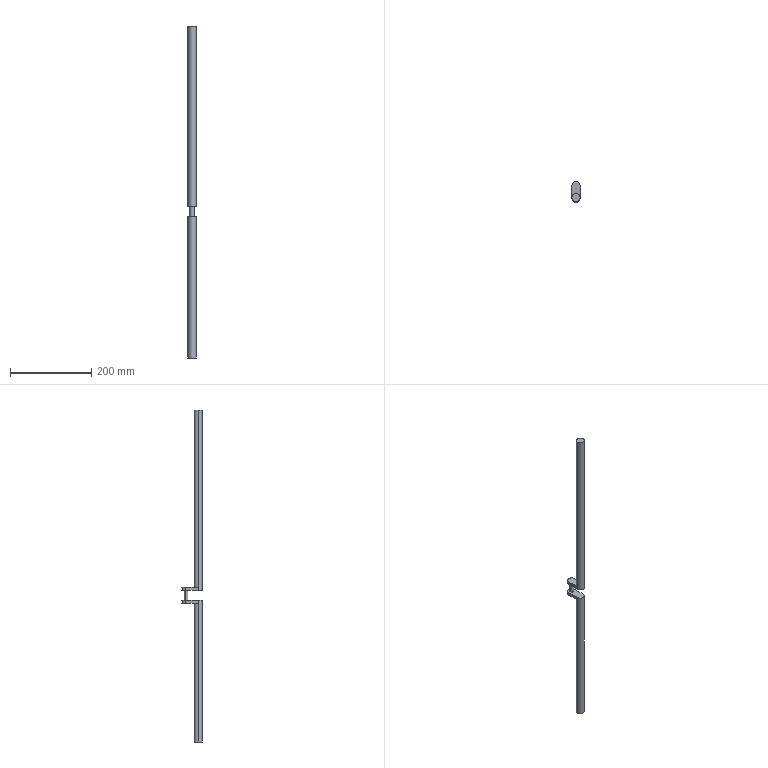Part | SolidWorks | features ICE 5, Extrusion 1 | 1 solid | 18 faces | box 20 x 50 x 819.2 mm | volume 260469 mm3 | plane 10 | cylinder 8 | commonest cylinder face diameters 20 x6 10 x2
STEP:
#1=CARTESIAN_POINT('',(10.,0.,457.2));
#2=VERTEX_POINT('',#1);
#3=CARTESIAN_POINT('',(-10.,0.,457.2));
#4=VERTEX_POINT('',#3);
#5=CARTESIAN_POINT('',(0.,0.,457.2));
#6=DIRECTION('',(0.,0.,1.));
#7=DIRECTION('',(1.,0.,0.));
#8=AXIS2_PLACEMENT_3D('',#5,#6,#7);
#9=CIRCLE('',#8,10.);
#10=EDGE_CURVE('',#2,#4,#9,.T.);
#11=ORIENTED_EDGE('',*,*,#10,.F.);
#12=CARTESIAN_POINT('',(10.,0.,20.));
#13=VERTEX_POINT('',#12);
#14=CARTESIAN_POINT('',(10.,0.,362.));
#15=DIRECTION('',(0.,0.,-1.));
#16=VECTOR('',#15,1000.);
#17=LINE('',#14,#16);
#18=EDGE_CURVE('',#2,#13,#17,.T.);
#19=ORIENTED_EDGE('',*,*,#18,.T.);
#20=CARTESIAN_POINT('',(-10.,0.,20.));
#21=VERTEX_POINT('',#20);
#22=CARTESIAN_POINT('',(0.,0.,20.));
#23=DIRECTION('',(0.,0.,1.));
#24=DIRECTION('',(1.,0.,0.));
#25=AXIS2_PLACEMENT_3D('',#22,#23,#24);
#26=CIRCLE('',#25,10.);
#27=EDGE_CURVE('',#13,#21,#26,.T.);
#28=ORIENTED_EDGE('',*,*,#27,.T.);
#29=CARTESIAN_POINT('',(-10.,0.,362.));
#30=DIRECTION('',(0.,0.,-1.));
#31=VECTOR('',#30,1000.);
#32=LINE('',#29,#31);
#33=EDGE_CURVE('',#4,#21,#32,.T.);
#34=ORIENTED_EDGE('',*,*,#33,.F.);
#35=EDGE_LOOP('',(#11,#19,#28,#34));
#36=FACE_OUTER_BOUND('',#35,.T.);
#37=CARTESIAN_POINT('',(0.,0.,362.));
#38=DIRECTION('',(0.,0.,-1.));
#39=DIRECTION('',(-1.,0.,0.));
#40=AXIS2_PLACEMENT_3D('',#37,#38,#39);
#41=CYLINDRICAL_SURFACE('',#40,10.);
#42=ADVANCED_FACE('',(#36),#41,.T.);
#43=CARTESIAN_POINT('',(5.,30.,12.5));
#44=VERTEX_POINT('',#43);
#45=CARTESIAN_POINT('',(-5.,30.,12.5));
#46=VERTEX_POINT('',#45);
#47=CARTESIAN_POINT('',(0.,30.,12.5));
#48=DIRECTION('',(0.,0.,1.));
#49=DIRECTION('',(1.,0.,0.));
#50=AXIS2_PLACEMENT_3D('',#47,#48,#49);
#51=CIRCLE('',#50,5.);
#52=EDGE_CURVE('',#44,#46,#51,.T.);
#53=ORIENTED_EDGE('',*,*,#52,.F.);
#54=CARTESIAN_POINT('',(5.,30.,-12.5));
#55=VERTEX_POINT('',#54);
#56=CARTESIAN_POINT('',(5.,30.,12.5));
#57=DIRECTION('',(0.,0.,-1.));
#58=VECTOR('',#57,1000.);
#59=LINE('',#56,#58);
#60=EDGE_CURVE('',#44,#55,#59,.T.);
#61=ORIENTED_EDGE('',*,*,#60,.T.);
#62=CARTESIAN_POINT('',(-5.,30.,-12.5));
#63=VERTEX_POINT('',#62);
#64=CARTESIAN_POINT('',(0.,30.,-12.5));
#65=DIRECTION('',(0.,0.,1.));
#66=DIRECTION('',(-1.,0.,0.));
#67=AXIS2_PLACEMENT_3D('',#64,#65,#66);
#68=CIRCLE('',#67,5.);
#69=EDGE_CURVE('',#55,#63,#68,.T.);
#70=ORIENTED_EDGE('',*,*,#69,.T.);
#71=CARTESIAN_POINT('',(-5.,30.,12.5));
#72=DIRECTION('',(0.,0.,-1.));
#73=VECTOR('',#72,1000.);
#74=LINE('',#71,#73);
#75=EDGE_CURVE('',#46,#63,#74,.T.);
#76=ORIENTED_EDGE('',*,*,#75,.F.);
#77=EDGE_LOOP('',(#53,#61,#70,#76));
#78=FACE_OUTER_BOUND('',#77,.T.);
#79=CARTESIAN_POINT('',(0.,30.,12.5));
#80=DIRECTION('',(0.,0.,-1.));
#81=DIRECTION('',(-1.,0.,0.));
#82=AXIS2_PLACEMENT_3D('',#79,#80,#81);
#83=CYLINDRICAL_SURFACE('',#82,5.);
#84=ADVANCED_FACE('',(#78),#83,.T.);
#85=CARTESIAN_POINT('',(-10.,0.,-20.));
#86=VERTEX_POINT('',#85);
#87=CARTESIAN_POINT('',(10.,0.,-20.));
#88=VERTEX_POINT('',#87);
#89=CARTESIAN_POINT('',(0.,0.,-20.));
#90=DIRECTION('',(0.,0.,-1.));
#91=DIRECTION('',(-1.,0.,0.));
#92=AXIS2_PLACEMENT_3D('',#89,#90,#91);
#93=CIRCLE('',#92,10.);
#94=EDGE_CURVE('',#86,#88,#93,.T.);
#95=ORIENTED_EDGE('',*,*,#94,.T.);
#96=CARTESIAN_POINT('',(10.,0.,-362.));
#97=VERTEX_POINT('',#96);
#98=CARTESIAN_POINT('',(10.,0.,362.));
#99=DIRECTION('',(0.,0.,-1.));
#100=VECTOR('',#99,1000.);
#101=LINE('',#98,#100);
#102=EDGE_CURVE('',#88,#97,#101,.T.);
#103=ORIENTED_EDGE('',*,*,#102,.T.);
#104=CARTESIAN_POINT('',(-10.,0.,-362.));
#105=VERTEX_POINT('',#104);
#106=CARTESIAN_POINT('',(0.,0.,-362.));
#107=DIRECTION('',(0.,0.,1.));
#108=DIRECTION('',(1.,0.,0.));
#109=AXIS2_PLACEMENT_3D('',#106,#107,#108);
#110=CIRCLE('',#109,10.);
#111=EDGE_CURVE('',#97,#105,#110,.T.);
#112=ORIENTED_EDGE('',*,*,#111,.T.);
#113=CARTESIAN_POINT('',(-10.,0.,362.));
#114=DIRECTION('',(0.,0.,-1.));
#115=VECTOR('',#114,1000.);
#116=LINE('',#113,#115);
#117=EDGE_CURVE('',#86,#105,#116,.T.);
#118=ORIENTED_EDGE('',*,*,#117,.F.);
#119=EDGE_LOOP('',(#95,#103,#112,#118));
#120=FACE_OUTER_BOUND('',#119,.T.);
#121=CARTESIAN_POINT('',(0.,0.,362.));
#122=DIRECTION('',(0.,0.,-1.));
#123=DIRECTION('',(-1.,0.,0.));
#124=AXIS2_PLACEMENT_3D('',#121,#122,#123);
#125=CYLINDRICAL_SURFACE('',#124,10.);
#126=ADVANCED_FACE('',(#120),#125,.T.);
#127=ORIENTED_EDGE('',*,*,#102,.F.);
#128=CARTESIAN_POINT('',(10.,0.,-12.5));
#129=VERTEX_POINT('',#128);
#130=CARTESIAN_POINT('',(10.,0.,20.));
#131=DIRECTION('',(0.,0.,-1.));
#132=VECTOR('',#131,1000.);
#133=LINE('',#130,#132);
#134=EDGE_CURVE('',#129,#88,#133,.T.);
#135=ORIENTED_EDGE('',*,*,#134,.F.);
#136=CARTESIAN_POINT('',(-10.,0.,-12.5));
#137=VERTEX_POINT('',#136);
#138=CARTESIAN_POINT('',(0.,0.,-12.5));
#139=DIRECTION('',(0.,0.,-1.));
#140=DIRECTION('',(-1.,0.,0.));
#141=AXIS2_PLACEMENT_3D('',#138,#139,#140);
#142=CIRCLE('',#141,10.);
#143=EDGE_CURVE('',#129,#137,#142,.T.);
#144=ORIENTED_EDGE('',*,*,#143,.T.);
#145=CARTESIAN_POINT('',(-10.,0.,20.));
#146=DIRECTION('',(0.,0.,-1.));
#147=VECTOR('',#146,1000.);
#148=LINE('',#145,#147);
#149=EDGE_CURVE('',#137,#86,#148,.T.);
#150=ORIENTED_EDGE('',*,*,#149,.T.);
#151=ORIENTED_EDGE('',*,*,#117,.T.);
#152=CARTESIAN_POINT('',(0.,0.,-362.));
#153=DIRECTION('',(0.,0.,1.));
#154=DIRECTION('',(1.,0.,0.));
#155=AXIS2_PLACEMENT_3D('',#152,#153,#154);
#156=CIRCLE('',#155,10.);
#157=EDGE_CURVE('',#105,#97,#156,.T.);
#158=ORIENTED_EDGE('',*,*,#157,.T.);
#159=EDGE_LOOP('',(#127,#135,#144,#150,#151,#158));
#160=FACE_OUTER_BOUND('',#159,.T.);
#161=CARTESIAN_POINT('',(0.,0.,362.));
#162=DIRECTION('',(0.,0.,-1.));
#163=DIRECTION('',(-1.,0.,0.));
#164=AXIS2_PLACEMENT_3D('',#161,#162,#163);
#165=CYLINDRICAL_SURFACE('',#164,10.);
#166=ADVANCED_FACE('',(#160),#165,.T.);
#167=CARTESIAN_POINT('',(10.,30.,-12.5));
#168=VERTEX_POINT('',#167);
#169=CARTESIAN_POINT('',(10.,30.,-20.));
#170=VERTEX_POINT('',#169);
#171=CARTESIAN_POINT('',(10.,30.,20.));
#172=DIRECTION('',(0.,0.,-1.));
#173=VECTOR('',#172,1000.);
#174=LINE('',#171,#173);
#175=EDGE_CURVE('',#168,#170,#174,.T.);
#176=ORIENTED_EDGE('',*,*,#175,.F.);
#177=CARTESIAN_POINT('',(10.,0.,-12.5));
#178=DIRECTION('',(0.,-1.,0.));
#179=VECTOR('',#178,1000.);
#180=LINE('',#177,#179);
#181=EDGE_CURVE('',#168,#129,#180,.T.);
#182=ORIENTED_EDGE('',*,*,#181,.T.);
#183=ORIENTED_EDGE('',*,*,#134,.T.);
#184=CARTESIAN_POINT('',(10.,0.,-20.));
#185=DIRECTION('',(0.,1.,0.));
#186=VECTOR('',#185,1000.);
#187=LINE('',#184,#186);
#188=EDGE_CURVE('',#88,#170,#187,.T.);
#189=ORIENTED_EDGE('',*,*,#188,.T.);
#190=EDGE_LOOP('',(#176,#182,#183,#189));
#191=FACE_OUTER_BOUND('',#190,.T.);
#192=CARTESIAN_POINT('',(10.,0.,20.));
#193=DIRECTION('',(-1.,0.,0.));
#194=DIRECTION('',(0.,0.,1.));
#195=AXIS2_PLACEMENT_3D('',#192,#193,#194);
#196=PLANE('',#195);
#197=ADVANCED_FACE('',(#191),#196,.F.);
#198=CARTESIAN_POINT('',(-10.,30.,-12.5));
#199=VERTEX_POINT('',#198);
#200=CARTESIAN_POINT('',(-10.,30.,-20.));
#201=VERTEX_POINT('',#200);
#202=CARTESIAN_POINT('',(-10.,30.,20.));
#203=DIRECTION('',(0.,0.,-1.));
#204=VECTOR('',#203,1000.);
#205=LINE('',#202,#204);
#206=EDGE_CURVE('',#199,#201,#205,.T.);
#207=ORIENTED_EDGE('',*,*,#206,.F.);
#208=CARTESIAN_POINT('',(0.,30.,-12.5));
#209=DIRECTION('',(0.,0.,-1.));
#210=DIRECTION('',(-1.,0.,0.));
#211=AXIS2_PLACEMENT_3D('',#208,#209,#210);
#212=CIRCLE('',#211,10.);
#213=EDGE_CURVE('',#199,#168,#212,.T.);
#214=ORIENTED_EDGE('',*,*,#213,.T.);
#215=ORIENTED_EDGE('',*,*,#175,.T.);
#216=CARTESIAN_POINT('',(0.,30.,-20.));
#217=DIRECTION('',(0.,0.,1.));
#218=DIRECTION('',(1.,0.,0.));
#219=AXIS2_PLACEMENT_3D('',#216,#217,#218);
#220=CIRCLE('',#219,10.);
#221=EDGE_CURVE('',#170,#201,#220,.T.);
#222=ORIENTED_EDGE('',*,*,#221,.T.);
#223=EDGE_LOOP('',(#207,#214,#215,#222));
#224=FACE_OUTER_BOUND('',#223,.T.);
#225=CARTESIAN_POINT('',(0.,30.,20.));
#226=DIRECTION('',(0.,0.,-1.));
#227=DIRECTION('',(-1.,0.,0.));
#228=AXIS2_PLACEMENT_3D('',#225,#226,#227);
#229=CYLINDRICAL_SURFACE('',#228,10.);
#230=ADVANCED_FACE('',(#224),#229,.T.);
#231=ORIENTED_EDGE('',*,*,#149,.F.);
#232=CARTESIAN_POINT('',(-10.,0.,-12.5));
#233=DIRECTION('',(0.,1.,0.));
#234=VECTOR('',#233,1000.);
#235=LINE('',#232,#234);
#236=EDGE_CURVE('',#137,#199,#235,.T.);
#237=ORIENTED_EDGE('',*,*,#236,.T.);
#238=ORIENTED_EDGE('',*,*,#206,.T.);
#239=CARTESIAN_POINT('',(-10.,0.,-20.));
#240=DIRECTION('',(0.,-1.,0.));
#241=VECTOR('',#240,1000.);
#242=LINE('',#239,#241);
#243=EDGE_CURVE('',#201,#86,#242,.T.);
#244=ORIENTED_EDGE('',*,*,#243,.T.);
#245=EDGE_LOOP('',(#231,#237,#238,#244));
#246=FACE_OUTER_BOUND('',#245,.T.);
#247=CARTESIAN_POINT('',(-10.,0.,20.));
#248=DIRECTION('',(1.,0.,0.));
#249=DIRECTION('',(0.,0.,-1.));
#250=AXIS2_PLACEMENT_3D('',#247,#248,#249);
#251=PLANE('',#250);
#252=ADVANCED_FACE('',(#246),#251,.F.);
#253=ORIENTED_EDGE('',*,*,#94,.F.);
#254=ORIENTED_EDGE('',*,*,#243,.F.);
#255=ORIENTED_EDGE('',*,*,#221,.F.);
#256=ORIENTED_EDGE('',*,*,#188,.F.);
#257=EDGE_LOOP('',(#253,#254,#255,#256));
#258=FACE_OUTER_BOUND('',#257,.T.);
#259=CARTESIAN_POINT('',(0.,0.,-20.));
#260=DIRECTION('',(0.,0.,1.));
#261=DIRECTION('',(1.,0.,0.));
#262=AXIS2_PLACEMENT_3D('',#259,#260,#261);
#263=PLANE('',#262);
#264=ADVANCED_FACE('',(#258),#263,.F.);
#265=ORIENTED_EDGE('',*,*,#157,.F.);
#266=ORIENTED_EDGE('',*,*,#111,.F.);
#267=EDGE_LOOP('',(#265,#266));
#268=FACE_OUTER_BOUND('',#267,.T.);
#269=CARTESIAN_POINT('',(0.,0.,-362.));
#270=DIRECTION('',(0.,0.,1.));
#271=DIRECTION('',(1.,0.,0.));
#272=AXIS2_PLACEMENT_3D('',#269,#270,#271);
#273=PLANE('',#272);
#274=ADVANCED_FACE('',(#268),#273,.F.);
#275=CARTESIAN_POINT('',(0.,30.,-12.5));
#276=DIRECTION('',(0.,0.,1.));
#277=DIRECTION('',(-1.,0.,0.));
#278=AXIS2_PLACEMENT_3D('',#275,#276,#277);
#279=CIRCLE('',#278,5.);
#280=EDGE_CURVE('',#63,#55,#279,.T.);
#281=ORIENTED_EDGE('',*,*,#280,.F.);
#282=ORIENTED_EDGE('',*,*,#69,.F.);
#283=EDGE_LOOP('',(#281,#282));
#284=FACE_BOUND('',#283,.T.);
#285=ORIENTED_EDGE('',*,*,#181,.F.);
#286=ORIENTED_EDGE('',*,*,#213,.F.);
#287=ORIENTED_EDGE('',*,*,#236,.F.);
#288=ORIENTED_EDGE('',*,*,#143,.F.);
#289=EDGE_LOOP('',(#285,#286,#287,#288));
#290=FACE_OUTER_BOUND('',#289,.T.);
#291=CARTESIAN_POINT('',(-10.,105.481,-12.5));
#292=DIRECTION('',(0.,0.,-1.));
#293=DIRECTION('',(-1.,0.,0.));
#294=AXIS2_PLACEMENT_3D('',#291,#292,#293);
#295=PLANE('',#294);
#296=ADVANCED_FACE('',(#284,#290),#295,.F.);
#297=ORIENTED_EDGE('',*,*,#60,.F.);
#298=CARTESIAN_POINT('',(0.,30.,12.5));
#299=DIRECTION('',(0.,0.,1.));
#300=DIRECTION('',(1.,0.,0.));
#301=AXIS2_PLACEMENT_3D('',#298,#299,#300);
#302=CIRCLE('',#301,5.);
#303=EDGE_CURVE('',#46,#44,#302,.T.);
#304=ORIENTED_EDGE('',*,*,#303,.F.);
#305=ORIENTED_EDGE('',*,*,#75,.T.);
#306=ORIENTED_EDGE('',*,*,#280,.T.);
#307=EDGE_LOOP('',(#297,#304,#305,#306));
#308=FACE_OUTER_BOUND('',#307,.T.);
#309=CARTESIAN_POINT('',(0.,30.,12.5));
#310=DIRECTION('',(0.,0.,-1.));
#311=DIRECTION('',(-1.,0.,0.));
#312=AXIS2_PLACEMENT_3D('',#309,#310,#311);
#313=CYLINDRICAL_SURFACE('',#312,5.);
#314=ADVANCED_FACE('',(#308),#313,.T.);
#315=ORIENTED_EDGE('',*,*,#27,.F.);
#316=CARTESIAN_POINT('',(10.,30.,20.));
#317=VERTEX_POINT('',#316);
#318=CARTESIAN_POINT('',(10.,0.,20.));
#319=DIRECTION('',(0.,1.,0.));
#320=VECTOR('',#319,1000.);
#321=LINE('',#318,#320);
#322=EDGE_CURVE('',#13,#317,#321,.T.);
#323=ORIENTED_EDGE('',*,*,#322,.T.);
#324=CARTESIAN_POINT('',(-10.,30.,20.));
#325=VERTEX_POINT('',#324);
#326=CARTESIAN_POINT('',(0.,30.,20.));
#327=DIRECTION('',(0.,0.,1.));
#328=DIRECTION('',(1.,0.,0.));
#329=AXIS2_PLACEMENT_3D('',#326,#327,#328);
#330=CIRCLE('',#329,10.);
#331=EDGE_CURVE('',#317,#325,#330,.T.);
#332=ORIENTED_EDGE('',*,*,#331,.T.);
#333=CARTESIAN_POINT('',(-10.,0.,20.));
#334=DIRECTION('',(0.,-1.,0.));
#335=VECTOR('',#334,1000.);
#336=LINE('',#333,#335);
#337=EDGE_CURVE('',#325,#21,#336,.T.);
#338=ORIENTED_EDGE('',*,*,#337,.T.);
#339=EDGE_LOOP('',(#315,#323,#332,#338));
#340=FACE_OUTER_BOUND('',#339,.T.);
#341=CARTESIAN_POINT('',(0.,0.,20.));
#342=DIRECTION('',(0.,0.,1.));
#343=DIRECTION('',(1.,0.,0.));
#344=AXIS2_PLACEMENT_3D('',#341,#342,#343);
#345=PLANE('',#344);
#346=ADVANCED_FACE('',(#340),#345,.T.);
#347=CARTESIAN_POINT('',(-10.,30.,12.5));
#348=VERTEX_POINT('',#347);
#349=CARTESIAN_POINT('',(-10.,30.,20.));
#350=DIRECTION('',(0.,0.,-1.));
#351=VECTOR('',#350,1000.);
#352=LINE('',#349,#351);
#353=EDGE_CURVE('',#325,#348,#352,.T.);
#354=ORIENTED_EDGE('',*,*,#353,.T.);
#355=CARTESIAN_POINT('',(-10.,0.,12.5));
#356=VERTEX_POINT('',#355);
#357=CARTESIAN_POINT('',(-10.,0.,12.5));
#358=DIRECTION('',(0.,-1.,0.));
#359=VECTOR('',#358,1000.);
#360=LINE('',#357,#359);
#361=EDGE_CURVE('',#348,#356,#360,.T.);
#362=ORIENTED_EDGE('',*,*,#361,.T.);
#363=CARTESIAN_POINT('',(-10.,0.,20.));
#364=DIRECTION('',(0.,0.,-1.));
#365=VECTOR('',#364,1000.);
#366=LINE('',#363,#365);
#367=EDGE_CURVE('',#21,#356,#366,.T.);
#368=ORIENTED_EDGE('',*,*,#367,.F.);
#369=ORIENTED_EDGE('',*,*,#337,.F.);
#370=EDGE_LOOP('',(#354,#362,#368,#369));
#371=FACE_OUTER_BOUND('',#370,.T.);
#372=CARTESIAN_POINT('',(-10.,0.,20.));
#373=DIRECTION('',(1.,0.,0.));
#374=DIRECTION('',(0.,0.,-1.));
#375=AXIS2_PLACEMENT_3D('',#372,#373,#374);
#376=PLANE('',#375);
#377=ADVANCED_FACE('',(#371),#376,.F.);
#378=CARTESIAN_POINT('',(10.,30.,12.5));
#379=VERTEX_POINT('',#378);
#380=CARTESIAN_POINT('',(10.,30.,20.));
#381=DIRECTION('',(0.,0.,-1.));
#382=VECTOR('',#381,1000.);
#383=LINE('',#380,#382);
#384=EDGE_CURVE('',#317,#379,#383,.T.);
#385=ORIENTED_EDGE('',*,*,#384,.T.);
#386=CARTESIAN_POINT('',(0.,30.,12.5));
#387=DIRECTION('',(0.,0.,1.));
#388=DIRECTION('',(1.,0.,0.));
#389=AXIS2_PLACEMENT_3D('',#386,#387,#388);
#390=CIRCLE('',#389,10.);
#391=EDGE_CURVE('',#379,#348,#390,.T.);
#392=ORIENTED_EDGE('',*,*,#391,.T.);
#393=ORIENTED_EDGE('',*,*,#353,.F.);
#394=ORIENTED_EDGE('',*,*,#331,.F.);
#395=EDGE_LOOP('',(#385,#392,#393,#394));
#396=FACE_OUTER_BOUND('',#395,.T.);
#397=CARTESIAN_POINT('',(0.,30.,20.));
#398=DIRECTION('',(0.,0.,-1.));
#399=DIRECTION('',(-1.,0.,0.));
#400=AXIS2_PLACEMENT_3D('',#397,#398,#399);
#401=CYLINDRICAL_SURFACE('',#400,10.);
#402=ADVANCED_FACE('',(#396),#401,.T.);
#403=CARTESIAN_POINT('',(10.,0.,12.5));
#404=VERTEX_POINT('',#403);
#405=CARTESIAN_POINT('',(10.,0.,20.));
#406=DIRECTION('',(0.,0.,-1.));
#407=VECTOR('',#406,1000.);
#408=LINE('',#405,#407);
#409=EDGE_CURVE('',#13,#404,#408,.T.);
#410=ORIENTED_EDGE('',*,*,#409,.T.);
#411=CARTESIAN_POINT('',(10.,0.,12.5));
#412=DIRECTION('',(0.,1.,0.));
#413=VECTOR('',#412,1000.);
#414=LINE('',#411,#413);
#415=EDGE_CURVE('',#404,#379,#414,.T.);
#416=ORIENTED_EDGE('',*,*,#415,.T.);
#417=ORIENTED_EDGE('',*,*,#384,.F.);
#418=ORIENTED_EDGE('',*,*,#322,.F.);
#419=EDGE_LOOP('',(#410,#416,#417,#418));
#420=FACE_OUTER_BOUND('',#419,.T.);
#421=CARTESIAN_POINT('',(10.,0.,20.));
#422=DIRECTION('',(-1.,0.,0.));
#423=DIRECTION('',(0.,0.,1.));
#424=AXIS2_PLACEMENT_3D('',#421,#422,#423);
#425=PLANE('',#424);
#426=ADVANCED_FACE('',(#420),#425,.F.);
#427=ORIENTED_EDGE('',*,*,#18,.F.);
#428=CARTESIAN_POINT('',(0.,0.,457.2));
#429=DIRECTION('',(0.,0.,1.));
#430=DIRECTION('',(1.,0.,0.));
#431=AXIS2_PLACEMENT_3D('',#428,#429,#430);
#432=CIRCLE('',#431,10.);
#433=EDGE_CURVE('',#4,#2,#432,.T.);
#434=ORIENTED_EDGE('',*,*,#433,.F.);
#435=ORIENTED_EDGE('',*,*,#33,.T.);
#436=ORIENTED_EDGE('',*,*,#367,.T.);
#437=CARTESIAN_POINT('',(0.,0.,12.5));
#438=DIRECTION('',(0.,0.,1.));
#439=DIRECTION('',(1.,0.,0.));
#440=AXIS2_PLACEMENT_3D('',#437,#438,#439);
#441=CIRCLE('',#440,10.);
#442=EDGE_CURVE('',#356,#404,#441,.T.);
#443=ORIENTED_EDGE('',*,*,#442,.T.);
#444=ORIENTED_EDGE('',*,*,#409,.F.);
#445=EDGE_LOOP('',(#427,#434,#435,#436,#443,#444));
#446=FACE_OUTER_BOUND('',#445,.T.);
#447=CARTESIAN_POINT('',(0.,0.,362.));
#448=DIRECTION('',(0.,0.,-1.));
#449=DIRECTION('',(-1.,0.,0.));
#450=AXIS2_PLACEMENT_3D('',#447,#448,#449);
#451=CYLINDRICAL_SURFACE('',#450,10.);
#452=ADVANCED_FACE('',(#446),#451,.T.);
#453=ORIENTED_EDGE('',*,*,#303,.T.);
#454=ORIENTED_EDGE('',*,*,#52,.T.);
#455=EDGE_LOOP('',(#453,#454));
#456=FACE_BOUND('',#455,.T.);
#457=ORIENTED_EDGE('',*,*,#361,.F.);
#458=ORIENTED_EDGE('',*,*,#391,.F.);
#459=ORIENTED_EDGE('',*,*,#415,.F.);
#460=ORIENTED_EDGE('',*,*,#442,.F.);
#461=EDGE_LOOP('',(#457,#458,#459,#460));
#462=FACE_OUTER_BOUND('',#461,.T.);
#463=CARTESIAN_POINT('',(-10.,105.481,12.5));
#464=DIRECTION('',(0.,0.,1.));
#465=DIRECTION('',(1.,0.,0.));
#466=AXIS2_PLACEMENT_3D('',#463,#464,#465);
#467=PLANE('',#466);
#468=ADVANCED_FACE('',(#456,#462),#467,.F.);
#469=ORIENTED_EDGE('',*,*,#433,.T.);
#470=ORIENTED_EDGE('',*,*,#10,.T.);
#471=EDGE_LOOP('',(#469,#470));
#472=FACE_OUTER_BOUND('',#471,.T.);
#473=CARTESIAN_POINT('',(0.,0.,457.2));
#474=DIRECTION('',(0.,0.,1.));
#475=DIRECTION('',(1.,0.,0.));
#476=AXIS2_PLACEMENT_3D('',#473,#474,#475);
#477=PLANE('',#476);
#478=ADVANCED_FACE('',(#472),#477,.T.);
#479=CLOSED_SHELL('',(#42,#84,#126,#166,#197,#230,#252,#264,#274,#296,#314,#346,#377,#402,#426,#452,#468,#478));
#480=MANIFOLD_SOLID_BREP('',#479);
#481=CARTESIAN_POINT('',(0.,0.,0.));
#482=DIRECTION('',(0.,0.,1.));
#483=DIRECTION('',(1.,0.,0.));
#484=AXIS2_PLACEMENT_3D('',#481,#482,#483);
#485=(LENGTH_UNIT()NAMED_UNIT(*)SI_UNIT(.MILLI.,.METRE.));
#486=UNCERTAINTY_MEASURE_WITH_UNIT(LENGTH_MEASURE(0.00001),#485,'','');
#487=(NAMED_UNIT(*)PLANE_ANGLE_UNIT()SI_UNIT($,.RADIAN.));
#488=(NAMED_UNIT(*)SI_UNIT($,.STERADIAN.)SOLID_ANGLE_UNIT());
#489=(GEOMETRIC_REPRESENTATION_CONTEXT(3)GLOBAL_UNCERTAINTY_ASSIGNED_CONTEXT((#486))GLOBAL_UNIT_ASSIGNED_CONTEXT((#485,#487,#488))REPRESENTATION_CONTEXT('',''));
#490=ADVANCED_BREP_SHAPE_REPRESENTATION('',(#480,#484),#489);